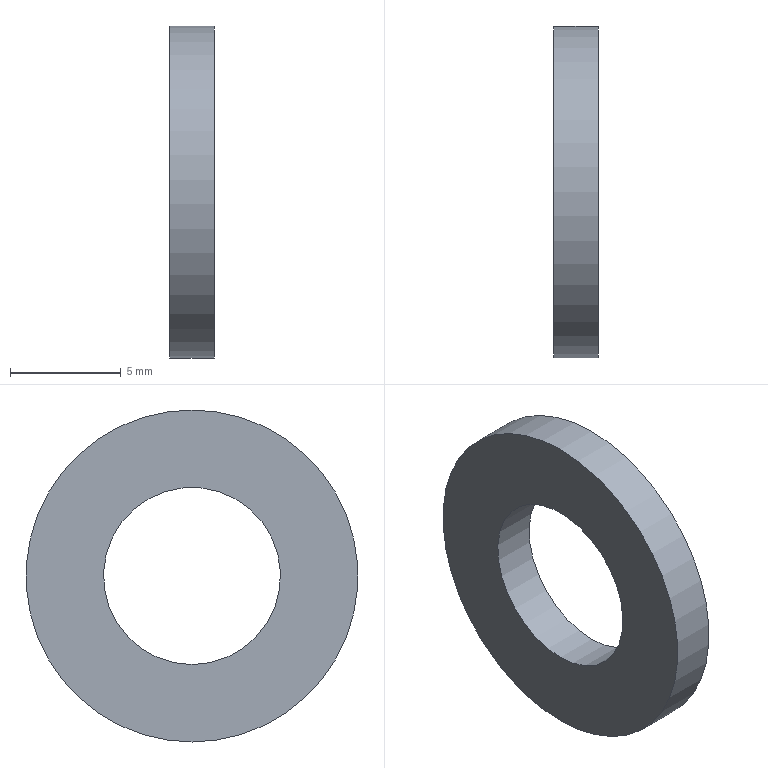Part | STEP file | Gasket [2] | 1 solid | 4 faces | box 2 x 15 x 15 mm | volume 252.898 mm3 | plane 2 | cylinder 2 | commonest cylinder face diameters 8 x1 15 x1
STEP:
#1=CARTESIAN_POINT('',(0.,0.,-7.5));
#2=VERTEX_POINT('',#1);
#3=CARTESIAN_POINT('',(0.,0.,0.));
#4=DIRECTION('',(1.,0.,0.));
#5=DIRECTION('',(0.,0.,-1.));
#6=AXIS2_PLACEMENT_3D('',#3,#4,#5);
#7=CIRCLE('',#6,7.5);
#8=EDGE_CURVE('',#2,#2,#7,.T.);
#9=ORIENTED_EDGE('',*,*,#8,.F.);
#10=EDGE_LOOP('',(#9));
#11=FACE_BOUND('',#10,.T.);
#12=CARTESIAN_POINT('',(0.,0.,-4.));
#13=VERTEX_POINT('',#12);
#14=CARTESIAN_POINT('',(0.,0.,0.));
#15=DIRECTION('',(1.,0.,0.));
#16=DIRECTION('',(0.,0.,-1.));
#17=AXIS2_PLACEMENT_3D('',#14,#15,#16);
#18=CIRCLE('',#17,4.);
#19=EDGE_CURVE('',#13,#13,#18,.T.);
#20=ORIENTED_EDGE('',*,*,#19,.T.);
#21=EDGE_LOOP('',(#20));
#22=FACE_BOUND('',#21,.T.);
#23=CARTESIAN_POINT('',(0.,0.,0.));
#24=DIRECTION('',(1.,0.,0.));
#25=DIRECTION('',(0.,0.,-1.));
#26=AXIS2_PLACEMENT_3D('',#23,#24,#25);
#27=PLANE('',#26);
#28=ADVANCED_FACE('',(#11,#22),#27,.F.);
#29=CARTESIAN_POINT('',(2.,0.,-7.5));
#30=VERTEX_POINT('',#29);
#31=CARTESIAN_POINT('',(2.,0.,0.));
#32=DIRECTION('',(1.,0.,0.));
#33=DIRECTION('',(0.,0.,-1.));
#34=AXIS2_PLACEMENT_3D('',#31,#32,#33);
#35=CIRCLE('',#34,7.5);
#36=EDGE_CURVE('',#30,#30,#35,.T.);
#37=ORIENTED_EDGE('',*,*,#36,.T.);
#38=EDGE_LOOP('',(#37));
#39=FACE_BOUND('',#38,.T.);
#40=CARTESIAN_POINT('',(2.,0.,-4.));
#41=VERTEX_POINT('',#40);
#42=CARTESIAN_POINT('',(2.,0.,0.));
#43=DIRECTION('',(1.,0.,0.));
#44=DIRECTION('',(0.,0.,-1.));
#45=AXIS2_PLACEMENT_3D('',#42,#43,#44);
#46=CIRCLE('',#45,4.);
#47=EDGE_CURVE('',#41,#41,#46,.F.);
#48=ORIENTED_EDGE('',*,*,#47,.T.);
#49=EDGE_LOOP('',(#48));
#50=FACE_BOUND('',#49,.T.);
#51=CARTESIAN_POINT('',(2.,0.,0.));
#52=DIRECTION('',(1.,0.,0.));
#53=DIRECTION('',(0.,0.,-1.));
#54=AXIS2_PLACEMENT_3D('',#51,#52,#53);
#55=PLANE('',#54);
#56=ADVANCED_FACE('',(#39,#50),#55,.T.);
#57=ORIENTED_EDGE('',*,*,#47,.F.);
#58=EDGE_LOOP('',(#57));
#59=FACE_OUTER_BOUND('',#58,.T.);
#60=ORIENTED_EDGE('',*,*,#19,.F.);
#61=EDGE_LOOP('',(#60));
#62=FACE_OUTER_BOUND('',#61,.T.);
#63=CARTESIAN_POINT('',(0.,0.,0.));
#64=DIRECTION('',(1.,0.,0.));
#65=DIRECTION('',(0.,0.,-1.));
#66=AXIS2_PLACEMENT_3D('',#63,#64,#65);
#67=CYLINDRICAL_SURFACE('',#66,4.);
#68=ADVANCED_FACE('',(#59,#62),#67,.F.);
#69=ORIENTED_EDGE('',*,*,#36,.F.);
#70=EDGE_LOOP('',(#69));
#71=FACE_OUTER_BOUND('',#70,.T.);
#72=ORIENTED_EDGE('',*,*,#8,.T.);
#73=EDGE_LOOP('',(#72));
#74=FACE_OUTER_BOUND('',#73,.T.);
#75=CARTESIAN_POINT('',(0.,0.,0.));
#76=DIRECTION('',(1.,0.,0.));
#77=DIRECTION('',(0.,0.,-1.));
#78=AXIS2_PLACEMENT_3D('',#75,#76,#77);
#79=CYLINDRICAL_SURFACE('',#78,7.5);
#80=ADVANCED_FACE('',(#71,#74),#79,.T.);
#81=CLOSED_SHELL('',(#28,#56,#68,#80));
#82=MANIFOLD_SOLID_BREP('',#81);
#83=(LENGTH_UNIT()NAMED_UNIT(*)SI_UNIT(.MILLI.,.METRE.));
#84=UNCERTAINTY_MEASURE_WITH_UNIT(LENGTH_MEASURE(0.00001),#83,'','');
#85=(NAMED_UNIT(*)PLANE_ANGLE_UNIT()SI_UNIT($,.RADIAN.));
#86=(NAMED_UNIT(*)SI_UNIT($,.STERADIAN.)SOLID_ANGLE_UNIT());
#87=(GEOMETRIC_REPRESENTATION_CONTEXT(3)GLOBAL_UNCERTAINTY_ASSIGNED_CONTEXT((#84))GLOBAL_UNIT_ASSIGNED_CONTEXT((#83,#85,#86))REPRESENTATION_CONTEXT('',''));
#88=ADVANCED_BREP_SHAPE_REPRESENTATION('',(#82),#87);